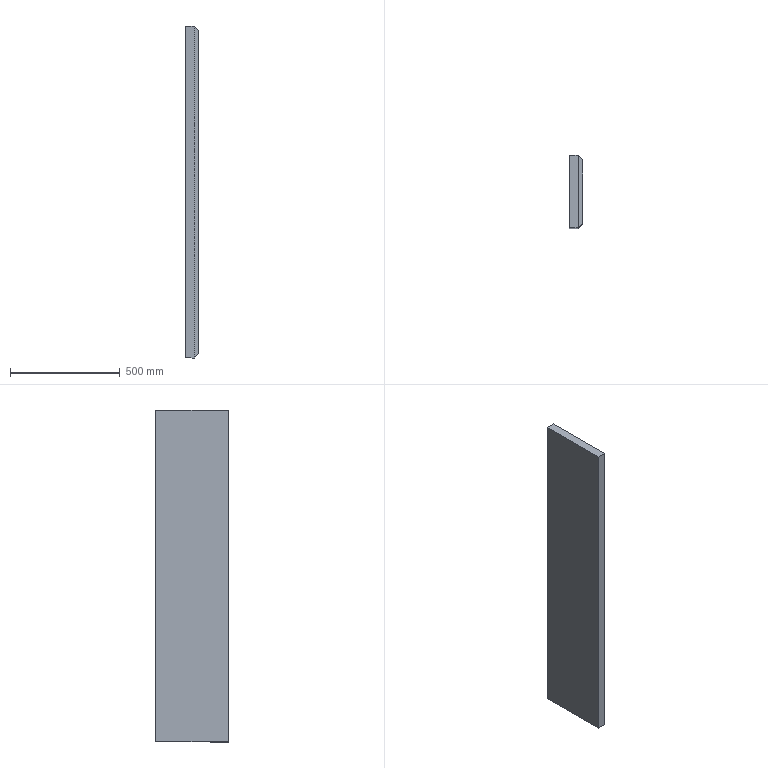Part | SolidWorks | features SplitBody 1 | 1 solid | 10 faces | box 60 x 330 x 1510 mm | volume 29172667 mm3 | plane 10
STEP:
#1=CARTESIAN_POINT('',(3261.,873.44,-755.));
#2=VERTEX_POINT('',#1);
#3=CARTESIAN_POINT('',(3261.,873.44,755.));
#4=VERTEX_POINT('',#3);
#5=CARTESIAN_POINT('',(3261.,873.44,755.));
#6=DIRECTION('',(0.,0.,1.));
#7=VECTOR('',#6,1000.);
#8=LINE('',#5,#7);
#9=EDGE_CURVE('',#2,#4,#8,.T.);
#10=ORIENTED_EDGE('',*,*,#9,.F.);
#11=CARTESIAN_POINT('',(3261.,543.44,-755.));
#12=VERTEX_POINT('',#11);
#13=CARTESIAN_POINT('',(3261.,543.44,-755.));
#14=DIRECTION('',(0.,1.,0.));
#15=VECTOR('',#14,1000.);
#16=LINE('',#13,#15);
#17=EDGE_CURVE('',#12,#2,#16,.T.);
#18=ORIENTED_EDGE('',*,*,#17,.F.);
#19=CARTESIAN_POINT('',(3261.,543.44,755.));
#20=VERTEX_POINT('',#19);
#21=CARTESIAN_POINT('',(3261.,543.44,755.));
#22=DIRECTION('',(0.,0.,-1.));
#23=VECTOR('',#22,1000.);
#24=LINE('',#21,#23);
#25=EDGE_CURVE('',#20,#12,#24,.T.);
#26=ORIENTED_EDGE('',*,*,#25,.F.);
#27=CARTESIAN_POINT('',(3261.,543.44,755.));
#28=DIRECTION('',(0.,-1.,0.));
#29=VECTOR('',#28,1000.);
#30=LINE('',#27,#29);
#31=EDGE_CURVE('',#4,#20,#30,.T.);
#32=ORIENTED_EDGE('',*,*,#31,.F.);
#33=EDGE_LOOP('',(#10,#18,#26,#32));
#34=FACE_OUTER_BOUND('',#33,.T.);
#35=CARTESIAN_POINT('',(3261.,543.44,755.));
#36=DIRECTION('',(1.,0.,0.));
#37=DIRECTION('',(0.,0.,-1.));
#38=AXIS2_PLACEMENT_3D('',#35,#36,#37);
#39=PLANE('',#38);
#40=ADVANCED_FACE('',(#34),#39,.F.);
#41=CARTESIAN_POINT('',(3301.,873.44,755.));
#42=VERTEX_POINT('',#41);
#43=CARTESIAN_POINT('',(3301.,543.44,755.));
#44=VERTEX_POINT('',#43);
#45=CARTESIAN_POINT('',(3301.,873.44,755.));
#46=DIRECTION('',(0.,-1.,0.));
#47=VECTOR('',#46,1000.);
#48=LINE('',#45,#47);
#49=EDGE_CURVE('',#42,#44,#48,.T.);
#50=ORIENTED_EDGE('',*,*,#49,.F.);
#51=CARTESIAN_POINT('',(3321.,873.44,755.));
#52=DIRECTION('',(1.,0.,0.));
#53=VECTOR('',#52,1000.);
#54=LINE('',#51,#53);
#55=EDGE_CURVE('',#4,#42,#54,.T.);
#56=ORIENTED_EDGE('',*,*,#55,.F.);
#57=ORIENTED_EDGE('',*,*,#31,.T.);
#58=CARTESIAN_POINT('',(3321.,543.44,755.));
#59=DIRECTION('',(-1.,0.,0.));
#60=VECTOR('',#59,1000.);
#61=LINE('',#58,#60);
#62=EDGE_CURVE('',#44,#20,#61,.T.);
#63=ORIENTED_EDGE('',*,*,#62,.F.);
#64=EDGE_LOOP('',(#50,#56,#57,#63));
#65=FACE_OUTER_BOUND('',#64,.T.);
#66=CARTESIAN_POINT('',(3321.,873.44,755.));
#67=DIRECTION('',(0.,0.,-1.));
#68=DIRECTION('',(0.,1.,0.));
#69=AXIS2_PLACEMENT_3D('',#66,#67,#68);
#70=PLANE('',#69);
#71=ADVANCED_FACE('',(#65),#70,.F.);
#72=CARTESIAN_POINT('',(3301.,873.44,-755.));
#73=VERTEX_POINT('',#72);
#74=CARTESIAN_POINT('',(3301.,873.44,755.));
#75=DIRECTION('',(0.,0.,1.));
#76=VECTOR('',#75,1000.);
#77=LINE('',#74,#76);
#78=EDGE_CURVE('',#73,#42,#77,.T.);
#79=ORIENTED_EDGE('',*,*,#78,.F.);
#80=CARTESIAN_POINT('',(3321.,873.44,-755.));
#81=DIRECTION('',(1.,0.,0.));
#82=VECTOR('',#81,1000.);
#83=LINE('',#80,#82);
#84=EDGE_CURVE('',#2,#73,#83,.T.);
#85=ORIENTED_EDGE('',*,*,#84,.F.);
#86=ORIENTED_EDGE('',*,*,#9,.T.);
#87=ORIENTED_EDGE('',*,*,#55,.T.);
#88=EDGE_LOOP('',(#79,#85,#86,#87));
#89=FACE_OUTER_BOUND('',#88,.T.);
#90=CARTESIAN_POINT('',(3321.,873.44,755.));
#91=DIRECTION('',(0.,-1.,0.));
#92=DIRECTION('',(-1.,0.,0.));
#93=AXIS2_PLACEMENT_3D('',#90,#91,#92);
#94=PLANE('',#93);
#95=ADVANCED_FACE('',(#89),#94,.F.);
#96=CARTESIAN_POINT('',(3301.,543.44,-755.));
#97=VERTEX_POINT('',#96);
#98=CARTESIAN_POINT('',(3301.,873.44,-755.));
#99=DIRECTION('',(0.,1.,0.));
#100=VECTOR('',#99,1000.);
#101=LINE('',#98,#100);
#102=EDGE_CURVE('',#97,#73,#101,.T.);
#103=ORIENTED_EDGE('',*,*,#102,.F.);
#104=CARTESIAN_POINT('',(3321.,543.44,-755.));
#105=DIRECTION('',(1.,0.,0.));
#106=VECTOR('',#105,1000.);
#107=LINE('',#104,#106);
#108=EDGE_CURVE('',#12,#97,#107,.T.);
#109=ORIENTED_EDGE('',*,*,#108,.F.);
#110=ORIENTED_EDGE('',*,*,#17,.T.);
#111=ORIENTED_EDGE('',*,*,#84,.T.);
#112=EDGE_LOOP('',(#103,#109,#110,#111));
#113=FACE_OUTER_BOUND('',#112,.T.);
#114=CARTESIAN_POINT('',(3321.,873.44,-755.));
#115=DIRECTION('',(0.,0.,1.));
#116=DIRECTION('',(1.,0.,0.));
#117=AXIS2_PLACEMENT_3D('',#114,#115,#116);
#118=PLANE('',#117);
#119=ADVANCED_FACE('',(#113),#118,.F.);
#120=CARTESIAN_POINT('',(3301.,543.44,755.));
#121=DIRECTION('',(0.,0.,-1.));
#122=VECTOR('',#121,1000.);
#123=LINE('',#120,#122);
#124=EDGE_CURVE('',#44,#97,#123,.T.);
#125=ORIENTED_EDGE('',*,*,#124,.F.);
#126=ORIENTED_EDGE('',*,*,#62,.T.);
#127=ORIENTED_EDGE('',*,*,#25,.T.);
#128=ORIENTED_EDGE('',*,*,#108,.T.);
#129=EDGE_LOOP('',(#125,#126,#127,#128));
#130=FACE_OUTER_BOUND('',#129,.T.);
#131=CARTESIAN_POINT('',(3321.,543.44,755.));
#132=DIRECTION('',(0.,1.,0.));
#133=DIRECTION('',(1.,0.,0.));
#134=AXIS2_PLACEMENT_3D('',#131,#132,#133);
#135=PLANE('',#134);
#136=ADVANCED_FACE('',(#130),#135,.F.);
#137=CARTESIAN_POINT('',(3321.,853.44,735.));
#138=VERTEX_POINT('',#137);
#139=CARTESIAN_POINT('',(3321.,853.44,735.));
#140=DIRECTION('',(-0.5774,0.5774,0.5774));
#141=VECTOR('',#140,1000.);
#142=LINE('',#139,#141);
#143=EDGE_CURVE('',#138,#42,#142,.T.);
#144=ORIENTED_EDGE('',*,*,#143,.T.);
#145=ORIENTED_EDGE('',*,*,#49,.T.);
#146=CARTESIAN_POINT('',(3321.,563.44,735.));
#147=VERTEX_POINT('',#146);
#148=CARTESIAN_POINT('',(3301.,543.44,755.));
#149=DIRECTION('',(0.5774,0.5774,-0.5774));
#150=VECTOR('',#149,1000.);
#151=LINE('',#148,#150);
#152=EDGE_CURVE('',#44,#147,#151,.T.);
#153=ORIENTED_EDGE('',*,*,#152,.T.);
#154=CARTESIAN_POINT('',(3321.,543.44,735.));
#155=DIRECTION('',(0.,1.,0.));
#156=VECTOR('',#155,1000.);
#157=LINE('',#154,#156);
#158=EDGE_CURVE('',#147,#138,#157,.T.);
#159=ORIENTED_EDGE('',*,*,#158,.T.);
#160=EDGE_LOOP('',(#144,#145,#153,#159));
#161=FACE_OUTER_BOUND('',#160,.T.);
#162=CARTESIAN_POINT('',(3321.,543.44,735.));
#163=DIRECTION('',(0.7071,0.,0.7071));
#164=DIRECTION('',(0.7071,0.,-0.7071));
#165=AXIS2_PLACEMENT_3D('',#162,#163,#164);
#166=PLANE('',#165);
#167=ADVANCED_FACE('',(#161),#166,.T.);
#168=ORIENTED_EDGE('',*,*,#143,.F.);
#169=CARTESIAN_POINT('',(3321.,853.44,-735.));
#170=VERTEX_POINT('',#169);
#171=CARTESIAN_POINT('',(3321.,853.44,755.));
#172=DIRECTION('',(0.,0.,-1.));
#173=VECTOR('',#172,1000.);
#174=LINE('',#171,#173);
#175=EDGE_CURVE('',#138,#170,#174,.T.);
#176=ORIENTED_EDGE('',*,*,#175,.T.);
#177=CARTESIAN_POINT('',(3321.,853.44,-735.));
#178=DIRECTION('',(-0.5774,0.5774,-0.5774));
#179=VECTOR('',#178,1000.);
#180=LINE('',#177,#179);
#181=EDGE_CURVE('',#170,#73,#180,.T.);
#182=ORIENTED_EDGE('',*,*,#181,.T.);
#183=ORIENTED_EDGE('',*,*,#78,.T.);
#184=EDGE_LOOP('',(#168,#176,#182,#183));
#185=FACE_OUTER_BOUND('',#184,.T.);
#186=CARTESIAN_POINT('',(3321.,853.44,755.));
#187=DIRECTION('',(0.7071,0.7071,0.));
#188=DIRECTION('',(0.7071,-0.7071,0.));
#189=AXIS2_PLACEMENT_3D('',#186,#187,#188);
#190=PLANE('',#189);
#191=ADVANCED_FACE('',(#185),#190,.T.);
#192=ORIENTED_EDGE('',*,*,#181,.F.);
#193=CARTESIAN_POINT('',(3321.,563.44,-735.));
#194=VERTEX_POINT('',#193);
#195=CARTESIAN_POINT('',(3321.,543.44,-735.));
#196=DIRECTION('',(0.,-1.,0.));
#197=VECTOR('',#196,1000.);
#198=LINE('',#195,#197);
#199=EDGE_CURVE('',#170,#194,#198,.T.);
#200=ORIENTED_EDGE('',*,*,#199,.T.);
#201=CARTESIAN_POINT('',(3321.,563.44,-735.));
#202=DIRECTION('',(-0.5774,-0.5774,-0.5774));
#203=VECTOR('',#202,1000.);
#204=LINE('',#201,#203);
#205=EDGE_CURVE('',#194,#97,#204,.T.);
#206=ORIENTED_EDGE('',*,*,#205,.T.);
#207=ORIENTED_EDGE('',*,*,#102,.T.);
#208=EDGE_LOOP('',(#192,#200,#206,#207));
#209=FACE_OUTER_BOUND('',#208,.T.);
#210=CARTESIAN_POINT('',(3321.,543.44,-735.));
#211=DIRECTION('',(0.7071,0.,-0.7071));
#212=DIRECTION('',(-0.7071,0.,-0.7071));
#213=AXIS2_PLACEMENT_3D('',#210,#211,#212);
#214=PLANE('',#213);
#215=ADVANCED_FACE('',(#209),#214,.T.);
#216=ORIENTED_EDGE('',*,*,#205,.F.);
#217=CARTESIAN_POINT('',(3321.,563.44,755.));
#218=DIRECTION('',(0.,0.,1.));
#219=VECTOR('',#218,1000.);
#220=LINE('',#217,#219);
#221=EDGE_CURVE('',#194,#147,#220,.T.);
#222=ORIENTED_EDGE('',*,*,#221,.T.);
#223=ORIENTED_EDGE('',*,*,#152,.F.);
#224=ORIENTED_EDGE('',*,*,#124,.T.);
#225=EDGE_LOOP('',(#216,#222,#223,#224));
#226=FACE_OUTER_BOUND('',#225,.T.);
#227=CARTESIAN_POINT('',(3321.,563.44,755.));
#228=DIRECTION('',(0.7071,-0.7071,0.));
#229=DIRECTION('',(-0.7071,-0.7071,0.));
#230=AXIS2_PLACEMENT_3D('',#227,#228,#229);
#231=PLANE('',#230);
#232=ADVANCED_FACE('',(#226),#231,.T.);
#233=ORIENTED_EDGE('',*,*,#158,.F.);
#234=ORIENTED_EDGE('',*,*,#221,.F.);
#235=ORIENTED_EDGE('',*,*,#199,.F.);
#236=ORIENTED_EDGE('',*,*,#175,.F.);
#237=EDGE_LOOP('',(#233,#234,#235,#236));
#238=FACE_OUTER_BOUND('',#237,.T.);
#239=CARTESIAN_POINT('',(3321.,543.44,755.));
#240=DIRECTION('',(1.,0.,0.));
#241=DIRECTION('',(0.,0.,-1.));
#242=AXIS2_PLACEMENT_3D('',#239,#240,#241);
#243=PLANE('',#242);
#244=ADVANCED_FACE('',(#238),#243,.T.);
#245=CLOSED_SHELL('',(#40,#71,#95,#119,#136,#167,#191,#215,#232,#244));
#246=MANIFOLD_SOLID_BREP('',#245);
#247=CARTESIAN_POINT('',(0.,0.,0.));
#248=DIRECTION('',(0.,0.,1.));
#249=DIRECTION('',(1.,0.,0.));
#250=AXIS2_PLACEMENT_3D('',#247,#248,#249);
#251=(LENGTH_UNIT()NAMED_UNIT(*)SI_UNIT(.MILLI.,.METRE.));
#252=UNCERTAINTY_MEASURE_WITH_UNIT(LENGTH_MEASURE(0.00001),#251,'','');
#253=(NAMED_UNIT(*)PLANE_ANGLE_UNIT()SI_UNIT($,.RADIAN.));
#254=(NAMED_UNIT(*)SI_UNIT($,.STERADIAN.)SOLID_ANGLE_UNIT());
#255=(GEOMETRIC_REPRESENTATION_CONTEXT(3)GLOBAL_UNCERTAINTY_ASSIGNED_CONTEXT((#252))GLOBAL_UNIT_ASSIGNED_CONTEXT((#251,#253,#254))REPRESENTATION_CONTEXT('',''));
#256=ADVANCED_BREP_SHAPE_REPRESENTATION('',(#246,#250),#255);